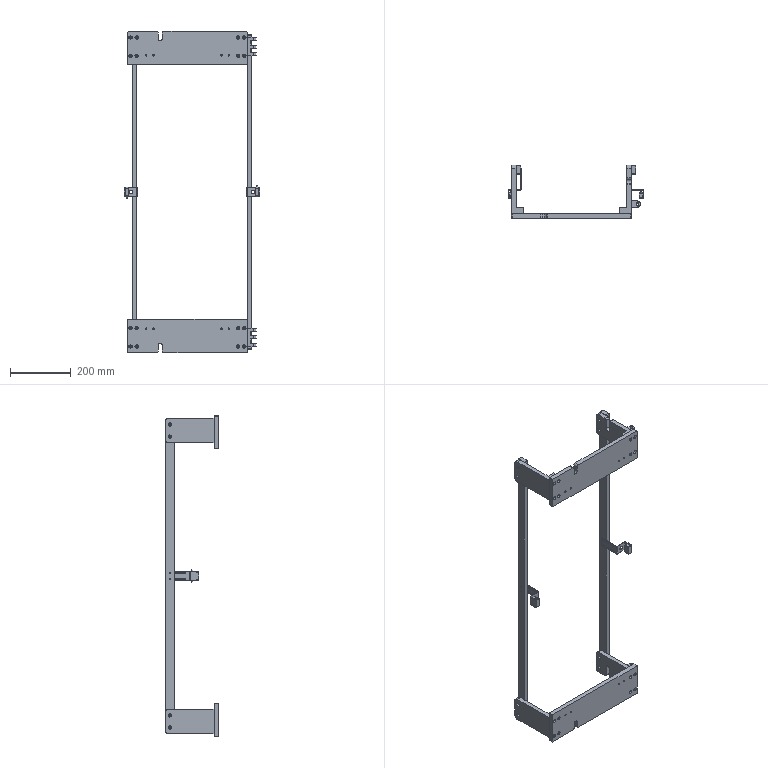Part | SolidWorks | 14 solids | 944 faces | box 445 x 175 x 1058 mm | volume 3157661 mm3 | cylinder 462 | plane 432 | cone 50 | commonest cylinder face diameters 5 x76 0.3 x50 11 x48 0.5 x44 6.4 x32 2.5 x20